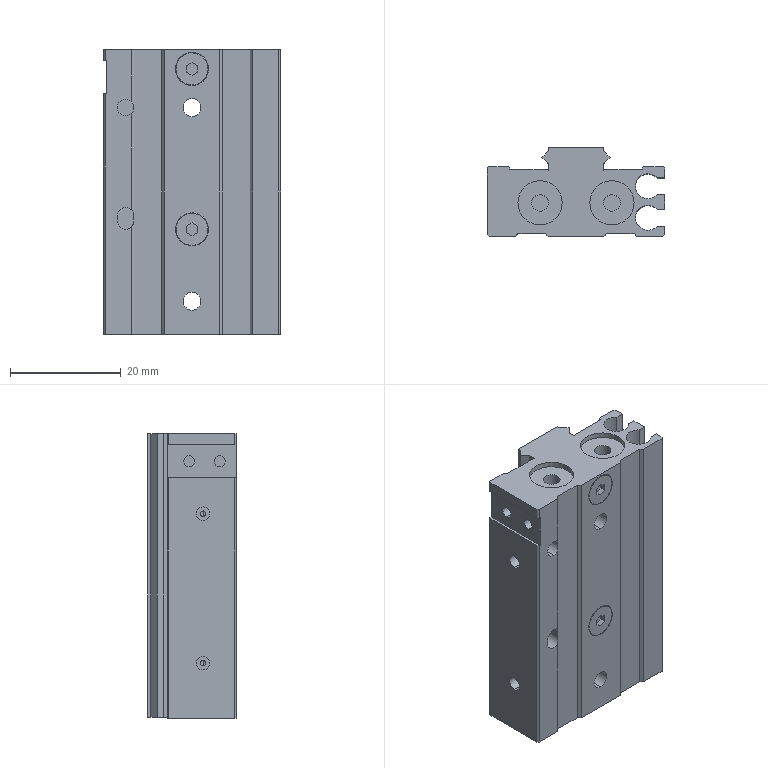Part | STEP file | QA-HI_MDX6x20-SG2BM2(0)_Bo | 1 solid | 153 faces | box 32 x 16 x 51.5 mm | volume 16782 mm3 | plane 92 | cylinder 57 | spline 4 | commonest cylinder face diameters 2.013 x12 3 x9 6 x8 8 x8 1 x4 2.459 x4